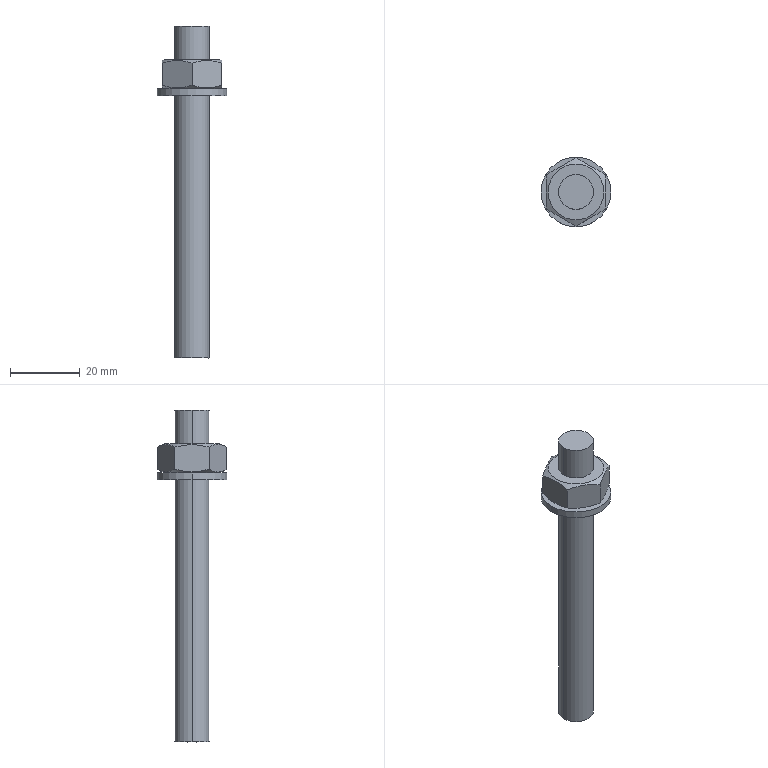Part | STEP file | PN_0013_bolt-type expansion anchor | 1 solid | 24 faces | box 20 x 20 x 95 mm | volume 9327 mm3 | plane 12 | cylinder 8 | cone 4 | commonest cylinder face diameters 10 x4 10.5 x2 20 x2